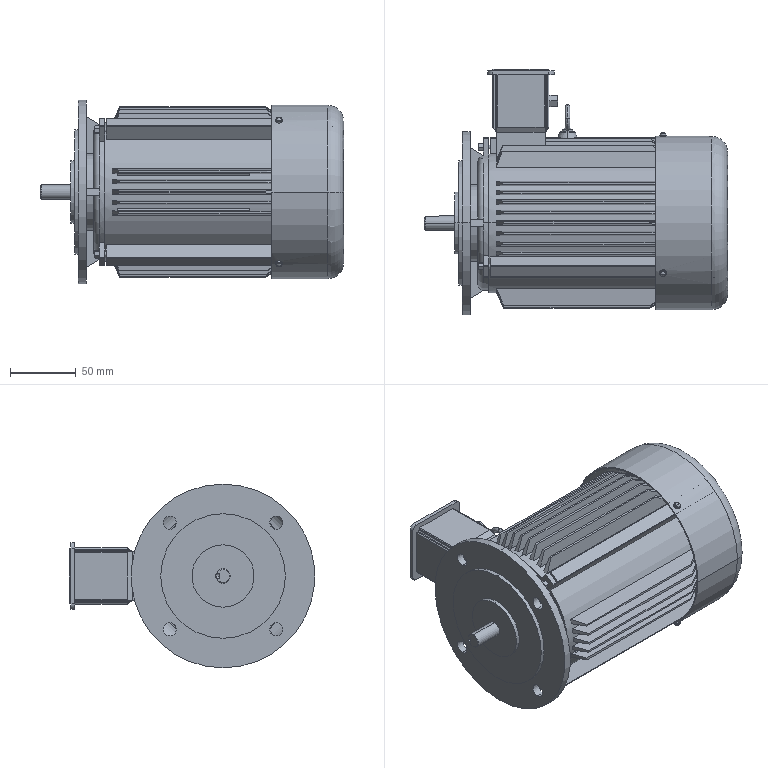Part | STEP file | Flanged end cover motor frame, no feet (TK) 63M | 1 solid | 448 faces | box 231 x 187 x 140 mm | volume 1853530 mm3 | plane 259 | cone 89 | cylinder 78 | torus 16 | sphere 6 | commonest cylinder face diameters 1.65 x12 8.25 x8 10 x8 3.25 x6 4.25 x6 5.25 x6